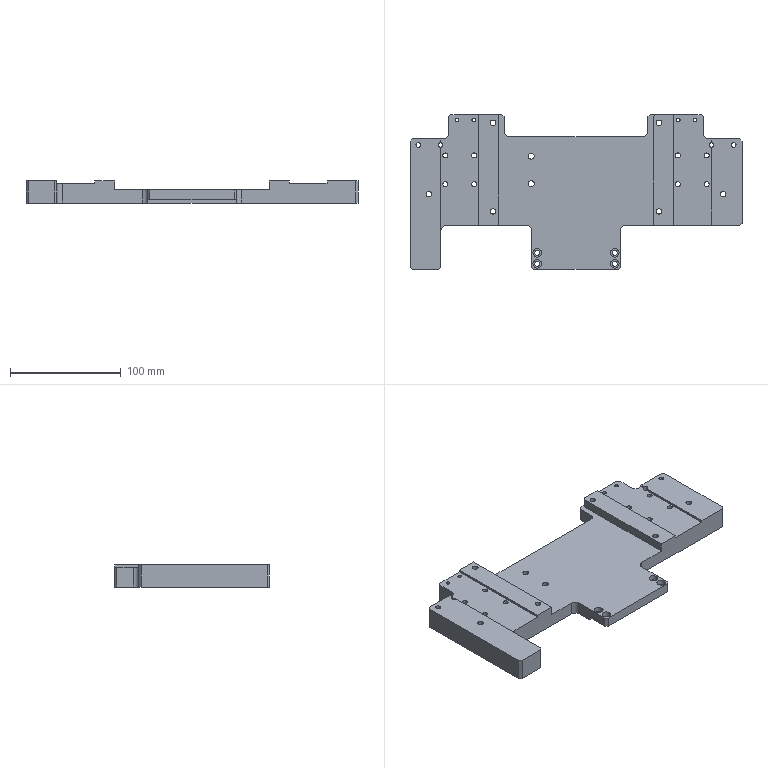Part | SolidWorks | features HoleWzd 8, Chamfer 5, Cut 4, Fillet 4, ICE 3, Extrusion 1 | 1 solid | 168 faces | box 300 x 140 x 20 mm | volume 458590 mm3 | cylinder 99 | plane 61 | cone 8 | commonest cylinder face diameters 4.5 x24 8 x16 5 x12 10 x11 2.5 x8 3.3 x8